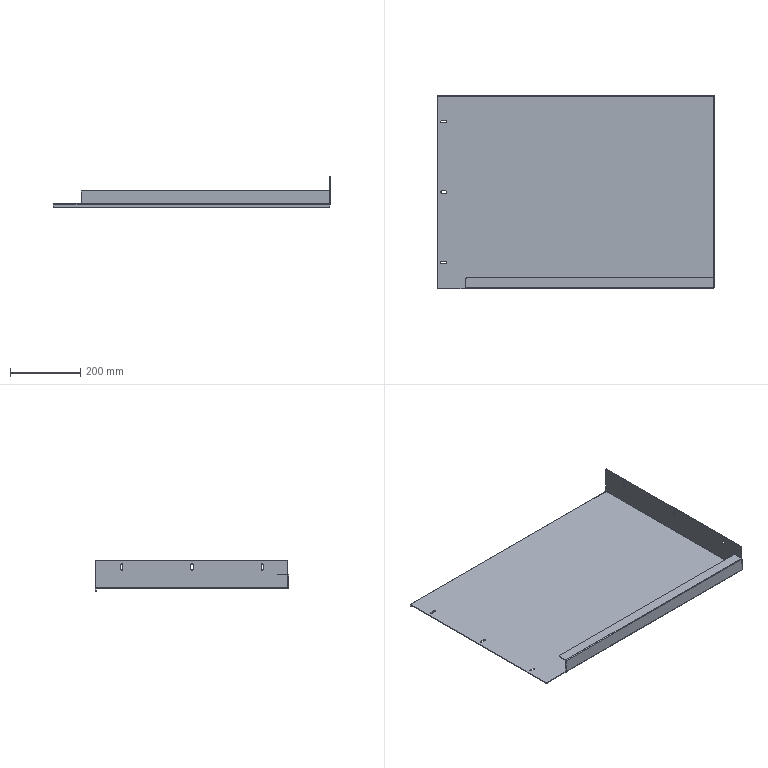Part | STEP file | 1 solid | 80 faces | box 790 x 550 x 88 mm | volume 1058095 mm3 | plane 45 | cylinder 33 | spline 2 | commonest cylinder face diameters 6 x25 0.2 x4 4.2 x4